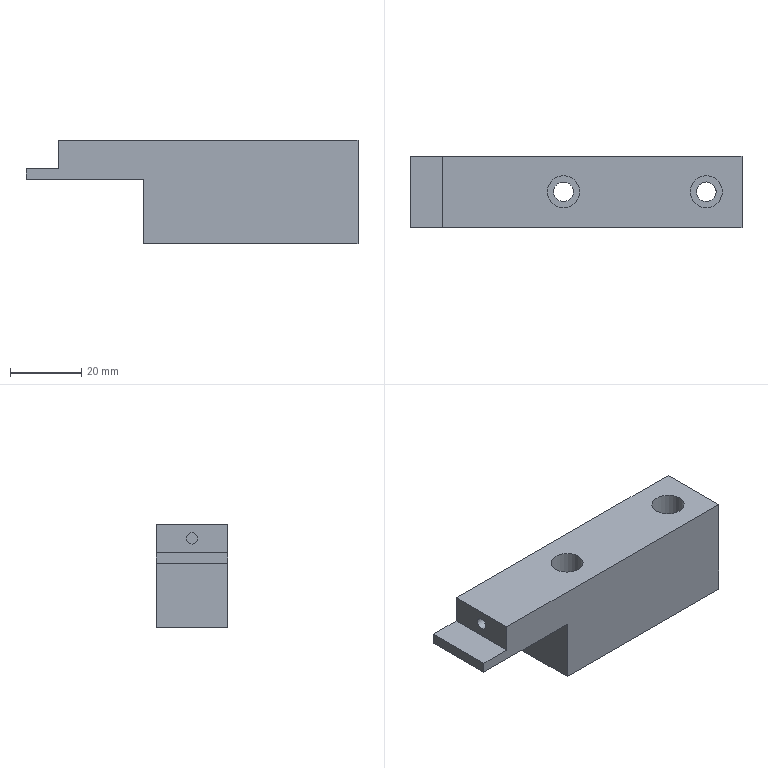Part | NX | 1 solid | 18 faces | box 93 x 20 x 29 mm | volume 38358 mm3 | plane 13 | cylinder 5 | commonest cylinder face diameters 5.5 x2 9 x2 3.2 x1
STEP:
#1=CARTESIAN_POINT('',(744.694,683.943,-134.9));
#2=VERTEX_POINT('',#1);
#3=CARTESIAN_POINT('',(744.694,683.943,-133.3));
#4=DIRECTION('',(1.,0.,0.));
#5=DIRECTION('',(0.,0.,-1.));
#6=AXIS2_PLACEMENT_3D('',#3,#4,#5);
#7=CIRCLE('',#6,1.6);
#8=EDGE_CURVE('',#2,#2,#7,.T.);
#9=ORIENTED_EDGE('',*,*,#8,.F.);
#10=EDGE_LOOP('',(#9));
#11=FACE_BOUND('',#10,.T.);
#12=CARTESIAN_POINT('',(754.694,683.943,-134.9));
#13=VERTEX_POINT('',#12);
#14=CARTESIAN_POINT('',(754.694,683.943,-133.3));
#15=DIRECTION('',(1.,0.,0.));
#16=DIRECTION('',(0.,0.,-1.));
#17=AXIS2_PLACEMENT_3D('',#14,#15,#16);
#18=CIRCLE('',#17,1.6);
#19=EDGE_CURVE('',#13,#13,#18,.T.);
#20=ORIENTED_EDGE('',*,*,#19,.T.);
#21=EDGE_LOOP('',(#20));
#22=FACE_BOUND('',#21,.T.);
#23=CARTESIAN_POINT('',(744.694,683.943,-133.3));
#24=DIRECTION('',(1.,0.,0.));
#25=DIRECTION('',(0.,0.,-1.));
#26=AXIS2_PLACEMENT_3D('',#23,#24,#25);
#27=CYLINDRICAL_SURFACE('',#26,1.6);
#28=ADVANCED_FACE('',(#11,#22),#27,.F.);
#29=ORIENTED_EDGE('',*,*,#19,.F.);
#30=EDGE_LOOP('',(#29));
#31=FACE_BOUND('',#30,.T.);
#32=CARTESIAN_POINT('',(754.694,683.943,-133.3));
#33=DIRECTION('',(1.,0.,0.));
#34=DIRECTION('',(0.,0.,-1.));
#35=AXIS2_PLACEMENT_3D('',#32,#33,#34);
#36=PLANE('',#35);
#37=ADVANCED_FACE('',(#31),#36,.F.);
#38=CARTESIAN_POINT('',(814.094,683.993,-129.35));
#39=VERTEX_POINT('',#38);
#40=CARTESIAN_POINT('',(818.594,683.993,-129.35));
#41=DIRECTION('',(0.,0.,-1.));
#42=DIRECTION('',(-1.,0.,0.));
#43=AXIS2_PLACEMENT_3D('',#40,#41,#42);
#44=CIRCLE('',#43,4.5);
#45=EDGE_CURVE('',#39,#39,#44,.T.);
#46=ORIENTED_EDGE('',*,*,#45,.F.);
#47=EDGE_LOOP('',(#46));
#48=FACE_BOUND('',#47,.T.);
#49=CARTESIAN_POINT('',(814.094,683.993,-139.35));
#50=VERTEX_POINT('',#49);
#51=CARTESIAN_POINT('',(818.594,683.993,-139.35));
#52=DIRECTION('',(0.,0.,-1.));
#53=DIRECTION('',(-1.,0.,0.));
#54=AXIS2_PLACEMENT_3D('',#51,#52,#53);
#55=CIRCLE('',#54,4.5);
#56=EDGE_CURVE('',#50,#50,#55,.T.);
#57=ORIENTED_EDGE('',*,*,#56,.T.);
#58=EDGE_LOOP('',(#57));
#59=FACE_BOUND('',#58,.T.);
#60=CARTESIAN_POINT('',(818.594,683.993,-129.35));
#61=DIRECTION('',(0.,0.,-1.));
#62=DIRECTION('',(-1.,0.,0.));
#63=AXIS2_PLACEMENT_3D('',#60,#61,#62);
#64=CYLINDRICAL_SURFACE('',#63,4.5);
#65=ADVANCED_FACE('',(#48,#59),#64,.F.);
#66=CARTESIAN_POINT('',(818.594,681.243,-139.35));
#67=VERTEX_POINT('',#66);
#68=CARTESIAN_POINT('',(818.594,683.993,-139.35));
#69=DIRECTION('',(0.,0.,1.));
#70=DIRECTION('',(0.,-1.,0.));
#71=AXIS2_PLACEMENT_3D('',#68,#69,#70);
#72=CIRCLE('',#71,2.75);
#73=EDGE_CURVE('',#67,#67,#72,.T.);
#74=ORIENTED_EDGE('',*,*,#73,.F.);
#75=EDGE_LOOP('',(#74));
#76=FACE_BOUND('',#75,.T.);
#77=ORIENTED_EDGE('',*,*,#56,.F.);
#78=EDGE_LOOP('',(#77));
#79=FACE_BOUND('',#78,.T.);
#80=CARTESIAN_POINT('',(818.594,683.993,-139.35));
#81=DIRECTION('',(0.,0.,-1.));
#82=DIRECTION('',(0.,-1.,0.));
#83=AXIS2_PLACEMENT_3D('',#80,#81,#82);
#84=PLANE('',#83);
#85=ADVANCED_FACE('',(#76,#79),#84,.F.);
#86=CARTESIAN_POINT('',(774.094,683.993,-129.35));
#87=VERTEX_POINT('',#86);
#88=CARTESIAN_POINT('',(778.594,683.993,-129.35));
#89=DIRECTION('',(0.,0.,-1.));
#90=DIRECTION('',(-1.,0.,0.));
#91=AXIS2_PLACEMENT_3D('',#88,#89,#90);
#92=CIRCLE('',#91,4.5);
#93=EDGE_CURVE('',#87,#87,#92,.T.);
#94=ORIENTED_EDGE('',*,*,#93,.F.);
#95=EDGE_LOOP('',(#94));
#96=FACE_BOUND('',#95,.T.);
#97=CARTESIAN_POINT('',(774.094,683.993,-139.35));
#98=VERTEX_POINT('',#97);
#99=CARTESIAN_POINT('',(778.594,683.993,-139.35));
#100=DIRECTION('',(0.,0.,-1.));
#101=DIRECTION('',(-1.,0.,0.));
#102=AXIS2_PLACEMENT_3D('',#99,#100,#101);
#103=CIRCLE('',#102,4.5);
#104=EDGE_CURVE('',#98,#98,#103,.T.);
#105=ORIENTED_EDGE('',*,*,#104,.T.);
#106=EDGE_LOOP('',(#105));
#107=FACE_BOUND('',#106,.T.);
#108=CARTESIAN_POINT('',(778.594,683.993,-129.35));
#109=DIRECTION('',(0.,0.,-1.));
#110=DIRECTION('',(-1.,0.,0.));
#111=AXIS2_PLACEMENT_3D('',#108,#109,#110);
#112=CYLINDRICAL_SURFACE('',#111,4.5);
#113=ADVANCED_FACE('',(#96,#107),#112,.F.);
#114=CARTESIAN_POINT('',(775.844,683.993,-139.35));
#115=VERTEX_POINT('',#114);
#116=CARTESIAN_POINT('',(778.594,683.993,-139.35));
#117=DIRECTION('',(0.,0.,1.));
#118=DIRECTION('',(-1.,0.,0.));
#119=AXIS2_PLACEMENT_3D('',#116,#117,#118);
#120=CIRCLE('',#119,2.75);
#121=EDGE_CURVE('',#115,#115,#120,.T.);
#122=ORIENTED_EDGE('',*,*,#121,.F.);
#123=EDGE_LOOP('',(#122));
#124=FACE_BOUND('',#123,.T.);
#125=ORIENTED_EDGE('',*,*,#104,.F.);
#126=EDGE_LOOP('',(#125));
#127=FACE_BOUND('',#126,.T.);
#128=CARTESIAN_POINT('',(818.594,683.993,-139.35));
#129=DIRECTION('',(0.,0.,-1.));
#130=DIRECTION('',(0.,-1.,0.));
#131=AXIS2_PLACEMENT_3D('',#128,#129,#130);
#132=PLANE('',#131);
#133=ADVANCED_FACE('',(#124,#127),#132,.F.);
#134=CARTESIAN_POINT('',(781.344,683.993,-158.35));
#135=VERTEX_POINT('',#134);
#136=CARTESIAN_POINT('',(778.594,683.993,-158.35));
#137=DIRECTION('',(0.,0.,-1.));
#138=DIRECTION('',(1.,0.,0.));
#139=AXIS2_PLACEMENT_3D('',#136,#137,#138);
#140=CIRCLE('',#139,2.75);
#141=EDGE_CURVE('',#135,#135,#140,.T.);
#142=ORIENTED_EDGE('',*,*,#141,.T.);
#143=EDGE_LOOP('',(#142));
#144=FACE_BOUND('',#143,.T.);
#145=ORIENTED_EDGE('',*,*,#121,.T.);
#146=EDGE_LOOP('',(#145));
#147=FACE_BOUND('',#146,.T.);
#148=CARTESIAN_POINT('',(778.594,683.993,-157.35));
#149=DIRECTION('',(0.,0.,1.));
#150=DIRECTION('',(1.,0.,0.));
#151=AXIS2_PLACEMENT_3D('',#148,#149,#150);
#152=CYLINDRICAL_SURFACE('',#151,2.75);
#153=ADVANCED_FACE('',(#144,#147),#152,.F.);
#154=CARTESIAN_POINT('',(821.344,683.993,-158.35));
#155=VERTEX_POINT('',#154);
#156=CARTESIAN_POINT('',(818.594,683.993,-158.35));
#157=DIRECTION('',(0.,0.,1.));
#158=DIRECTION('',(1.,0.,0.));
#159=AXIS2_PLACEMENT_3D('',#156,#157,#158);
#160=CIRCLE('',#159,2.75);
#161=EDGE_CURVE('',#155,#155,#160,.T.);
#162=ORIENTED_EDGE('',*,*,#161,.F.);
#163=EDGE_LOOP('',(#162));
#164=FACE_BOUND('',#163,.T.);
#165=ORIENTED_EDGE('',*,*,#73,.T.);
#166=EDGE_LOOP('',(#165));
#167=FACE_BOUND('',#166,.T.);
#168=CARTESIAN_POINT('',(818.594,683.993,-157.35));
#169=DIRECTION('',(0.,0.,1.));
#170=DIRECTION('',(-1.,0.,0.));
#171=AXIS2_PLACEMENT_3D('',#168,#169,#170);
#172=CYLINDRICAL_SURFACE('',#171,2.75);
#173=ADVANCED_FACE('',(#164,#167),#172,.F.);
#174=CARTESIAN_POINT('',(744.694,673.943,-129.35));
#175=VERTEX_POINT('',#174);
#176=CARTESIAN_POINT('',(744.694,673.943,-137.3));
#177=VERTEX_POINT('',#176);
#178=CARTESIAN_POINT('',(744.694,673.943,-129.35));
#179=DIRECTION('',(0.,0.,-1.));
#180=VECTOR('',#179,1000.);
#181=LINE('',#178,#180);
#182=EDGE_CURVE('',#175,#177,#181,.T.);
#183=ORIENTED_EDGE('',*,*,#182,.F.);
#184=CARTESIAN_POINT('',(744.694,693.943,-129.35));
#185=VERTEX_POINT('',#184);
#186=CARTESIAN_POINT('',(744.694,892.443,-129.35));
#187=DIRECTION('',(0.,-1.,0.));
#188=VECTOR('',#187,1000.);
#189=LINE('',#186,#188);
#190=EDGE_CURVE('',#185,#175,#189,.T.);
#191=ORIENTED_EDGE('',*,*,#190,.F.);
#192=CARTESIAN_POINT('',(744.694,693.943,-137.3));
#193=VERTEX_POINT('',#192);
#194=CARTESIAN_POINT('',(744.694,693.943,-129.35));
#195=DIRECTION('',(0.,0.,-1.));
#196=VECTOR('',#195,1000.);
#197=LINE('',#194,#196);
#198=EDGE_CURVE('',#185,#193,#197,.T.);
#199=ORIENTED_EDGE('',*,*,#198,.T.);
#200=CARTESIAN_POINT('',(744.694,892.443,-137.3));
#201=DIRECTION('',(0.,1.,0.));
#202=VECTOR('',#201,1000.);
#203=LINE('',#200,#202);
#204=EDGE_CURVE('',#177,#193,#203,.T.);
#205=ORIENTED_EDGE('',*,*,#204,.F.);
#206=EDGE_LOOP('',(#183,#191,#199,#205));
#207=FACE_BOUND('',#206,.T.);
#208=ORIENTED_EDGE('',*,*,#8,.T.);
#209=EDGE_LOOP('',(#208));
#210=FACE_BOUND('',#209,.T.);
#211=CARTESIAN_POINT('',(744.694,892.443,-139.3));
#212=DIRECTION('',(1.,0.,0.));
#213=DIRECTION('',(0.,1.,0.));
#214=AXIS2_PLACEMENT_3D('',#211,#212,#213);
#215=PLANE('',#214);
#216=ADVANCED_FACE('',(#207,#210),#215,.F.);
#217=CARTESIAN_POINT('',(768.594,693.943,-140.35));
#218=VERTEX_POINT('',#217);
#219=CARTESIAN_POINT('',(768.594,673.943,-140.35));
#220=VERTEX_POINT('',#219);
#221=CARTESIAN_POINT('',(768.594,605.243,-140.35));
#222=DIRECTION('',(0.,-1.,0.));
#223=VECTOR('',#222,1000.);
#224=LINE('',#221,#223);
#225=EDGE_CURVE('',#218,#220,#224,.T.);
#226=ORIENTED_EDGE('',*,*,#225,.F.);
#227=CARTESIAN_POINT('',(768.594,693.943,-158.35));
#228=VERTEX_POINT('',#227);
#229=CARTESIAN_POINT('',(768.594,693.943,-164.35));
#230=DIRECTION('',(0.,0.,-1.));
#231=VECTOR('',#230,1000.);
#232=LINE('',#229,#231);
#233=EDGE_CURVE('',#218,#228,#232,.T.);
#234=ORIENTED_EDGE('',*,*,#233,.T.);
#235=CARTESIAN_POINT('',(768.594,673.943,-158.35));
#236=VERTEX_POINT('',#235);
#237=CARTESIAN_POINT('',(768.594,605.243,-158.35));
#238=DIRECTION('',(0.,1.,0.));
#239=VECTOR('',#238,1000.);
#240=LINE('',#237,#239);
#241=EDGE_CURVE('',#236,#228,#240,.T.);
#242=ORIENTED_EDGE('',*,*,#241,.F.);
#243=CARTESIAN_POINT('',(768.594,673.943,-164.35));
#244=DIRECTION('',(0.,0.,-1.));
#245=VECTOR('',#244,1000.);
#246=LINE('',#243,#245);
#247=EDGE_CURVE('',#220,#236,#246,.T.);
#248=ORIENTED_EDGE('',*,*,#247,.F.);
#249=EDGE_LOOP('',(#226,#234,#242,#248));
#250=FACE_BOUND('',#249,.T.);
#251=CARTESIAN_POINT('',(768.594,605.243,-164.35));
#252=DIRECTION('',(-1.,0.,0.));
#253=DIRECTION('',(0.,-1.,0.));
#254=AXIS2_PLACEMENT_3D('',#251,#252,#253);
#255=PLANE('',#254);
#256=ADVANCED_FACE('',(#250),#255,.T.);
#257=ORIENTED_EDGE('',*,*,#241,.T.);
#258=CARTESIAN_POINT('',(828.594,693.943,-158.35));
#259=VERTEX_POINT('',#258);
#260=CARTESIAN_POINT('',(798.594,693.943,-158.35));
#261=DIRECTION('',(1.,0.,0.));
#262=VECTOR('',#261,1000.);
#263=LINE('',#260,#262);
#264=EDGE_CURVE('',#228,#259,#263,.T.);
#265=ORIENTED_EDGE('',*,*,#264,.T.);
#266=CARTESIAN_POINT('',(828.594,673.943,-158.35));
#267=VERTEX_POINT('',#266);
#268=CARTESIAN_POINT('',(828.594,605.243,-158.35));
#269=DIRECTION('',(0.,1.,0.));
#270=VECTOR('',#269,1000.);
#271=LINE('',#268,#270);
#272=EDGE_CURVE('',#267,#259,#271,.T.);
#273=ORIENTED_EDGE('',*,*,#272,.F.);
#274=CARTESIAN_POINT('',(798.594,673.943,-158.35));
#275=DIRECTION('',(1.,0.,0.));
#276=VECTOR('',#275,1000.);
#277=LINE('',#274,#276);
#278=EDGE_CURVE('',#236,#267,#277,.T.);
#279=ORIENTED_EDGE('',*,*,#278,.F.);
#280=EDGE_LOOP('',(#257,#265,#273,#279));
#281=FACE_BOUND('',#280,.T.);
#282=ORIENTED_EDGE('',*,*,#161,.T.);
#283=EDGE_LOOP('',(#282));
#284=FACE_BOUND('',#283,.T.);
#285=ORIENTED_EDGE('',*,*,#141,.F.);
#286=EDGE_LOOP('',(#285));
#287=FACE_BOUND('',#286,.T.);
#288=CARTESIAN_POINT('',(798.594,605.243,-158.35));
#289=DIRECTION('',(0.,0.,1.));
#290=DIRECTION('',(0.,1.,0.));
#291=AXIS2_PLACEMENT_3D('',#288,#289,#290);
#292=PLANE('',#291);
#293=ADVANCED_FACE('',(#281,#284,#287),#292,.F.);
#294=CARTESIAN_POINT('',(735.594,693.943,-137.3));
#295=VERTEX_POINT('',#294);
#296=CARTESIAN_POINT('',(830.394,693.943,-137.3));
#297=DIRECTION('',(-1.,0.,0.));
#298=VECTOR('',#297,1000.);
#299=LINE('',#296,#298);
#300=EDGE_CURVE('',#193,#295,#299,.T.);
#301=ORIENTED_EDGE('',*,*,#300,.T.);
#302=CARTESIAN_POINT('',(735.594,673.943,-137.3));
#303=VERTEX_POINT('',#302);
#304=CARTESIAN_POINT('',(735.594,717.943,-137.3));
#305=DIRECTION('',(0.,1.,0.));
#306=VECTOR('',#305,1000.);
#307=LINE('',#304,#306);
#308=EDGE_CURVE('',#303,#295,#307,.T.);
#309=ORIENTED_EDGE('',*,*,#308,.F.);
#310=CARTESIAN_POINT('',(830.394,673.943,-137.3));
#311=DIRECTION('',(-1.,0.,0.));
#312=VECTOR('',#311,1000.);
#313=LINE('',#310,#312);
#314=EDGE_CURVE('',#177,#303,#313,.T.);
#315=ORIENTED_EDGE('',*,*,#314,.F.);
#316=ORIENTED_EDGE('',*,*,#204,.T.);
#317=EDGE_LOOP('',(#301,#309,#315,#316));
#318=FACE_BOUND('',#317,.T.);
#319=CARTESIAN_POINT('',(743.694,717.943,-137.3));
#320=DIRECTION('',(0.,0.,-1.));
#321=DIRECTION('',(0.,-1.,0.));
#322=AXIS2_PLACEMENT_3D('',#319,#320,#321);
#323=PLANE('',#322);
#324=ADVANCED_FACE('',(#318),#323,.F.);
#325=CARTESIAN_POINT('',(828.594,673.943,-129.35));
#326=VERTEX_POINT('',#325);
#327=CARTESIAN_POINT('',(828.594,673.943,-129.35));
#328=DIRECTION('',(0.,0.,-1.));
#329=VECTOR('',#328,1000.);
#330=LINE('',#327,#329);
#331=EDGE_CURVE('',#326,#267,#330,.T.);
#332=ORIENTED_EDGE('',*,*,#331,.T.);
#333=ORIENTED_EDGE('',*,*,#272,.T.);
#334=CARTESIAN_POINT('',(828.594,693.943,-129.35));
#335=VERTEX_POINT('',#334);
#336=CARTESIAN_POINT('',(828.594,693.943,-164.35));
#337=DIRECTION('',(0.,0.,1.));
#338=VECTOR('',#337,1000.);
#339=LINE('',#336,#338);
#340=EDGE_CURVE('',#259,#335,#339,.T.);
#341=ORIENTED_EDGE('',*,*,#340,.T.);
#342=CARTESIAN_POINT('',(828.594,570.943,-129.35));
#343=DIRECTION('',(0.,1.,0.));
#344=VECTOR('',#343,1000.);
#345=LINE('',#342,#344);
#346=EDGE_CURVE('',#326,#335,#345,.T.);
#347=ORIENTED_EDGE('',*,*,#346,.F.);
#348=EDGE_LOOP('',(#332,#333,#341,#347));
#349=FACE_BOUND('',#348,.T.);
#350=CARTESIAN_POINT('',(828.594,605.243,-164.35));
#351=DIRECTION('',(1.,0.,0.));
#352=DIRECTION('',(0.,1.,0.));
#353=AXIS2_PLACEMENT_3D('',#350,#351,#352);
#354=PLANE('',#353);
#355=ADVANCED_FACE('',(#349),#354,.T.);
#356=CARTESIAN_POINT('',(830.394,673.943,-129.35));
#357=DIRECTION('',(1.,0.,0.));
#358=VECTOR('',#357,1000.);
#359=LINE('',#356,#358);
#360=EDGE_CURVE('',#175,#326,#359,.T.);
#361=ORIENTED_EDGE('',*,*,#360,.F.);
#362=ORIENTED_EDGE('',*,*,#182,.T.);
#363=ORIENTED_EDGE('',*,*,#314,.T.);
#364=CARTESIAN_POINT('',(735.594,673.943,-140.35));
#365=VERTEX_POINT('',#364);
#366=CARTESIAN_POINT('',(735.594,673.943,-139.3));
#367=DIRECTION('',(0.,0.,-1.));
#368=VECTOR('',#367,1000.);
#369=LINE('',#366,#368);
#370=EDGE_CURVE('',#303,#365,#369,.T.);
#371=ORIENTED_EDGE('',*,*,#370,.T.);
#372=CARTESIAN_POINT('',(740.194,673.943,-140.35));
#373=DIRECTION('',(1.,0.,0.));
#374=VECTOR('',#373,1000.);
#375=LINE('',#372,#374);
#376=EDGE_CURVE('',#365,#220,#375,.T.);
#377=ORIENTED_EDGE('',*,*,#376,.T.);
#378=ORIENTED_EDGE('',*,*,#247,.T.);
#379=ORIENTED_EDGE('',*,*,#278,.T.);
#380=ORIENTED_EDGE('',*,*,#331,.F.);
#381=EDGE_LOOP('',(#361,#362,#363,#371,#377,#378,#379,#380));
#382=FACE_BOUND('',#381,.T.);
#383=CARTESIAN_POINT('',(830.394,673.943,-129.35));
#384=DIRECTION('',(0.,1.,0.));
#385=DIRECTION('',(-1.,0.,0.));
#386=AXIS2_PLACEMENT_3D('',#383,#384,#385);
#387=PLANE('',#386);
#388=ADVANCED_FACE('',(#382),#387,.F.);
#389=ORIENTED_EDGE('',*,*,#300,.F.);
#390=ORIENTED_EDGE('',*,*,#198,.F.);
#391=CARTESIAN_POINT('',(830.394,693.943,-129.35));
#392=DIRECTION('',(1.,0.,0.));
#393=VECTOR('',#392,1000.);
#394=LINE('',#391,#393);
#395=EDGE_CURVE('',#185,#335,#394,.T.);
#396=ORIENTED_EDGE('',*,*,#395,.T.);
#397=ORIENTED_EDGE('',*,*,#340,.F.);
#398=ORIENTED_EDGE('',*,*,#264,.F.);
#399=ORIENTED_EDGE('',*,*,#233,.F.);
#400=CARTESIAN_POINT('',(735.594,693.943,-140.35));
#401=VERTEX_POINT('',#400);
#402=CARTESIAN_POINT('',(830.394,693.943,-140.35));
#403=DIRECTION('',(-1.,0.,0.));
#404=VECTOR('',#403,1000.);
#405=LINE('',#402,#404);
#406=EDGE_CURVE('',#218,#401,#405,.T.);
#407=ORIENTED_EDGE('',*,*,#406,.T.);
#408=CARTESIAN_POINT('',(735.594,693.943,-139.3));
#409=DIRECTION('',(0.,0.,-1.));
#410=VECTOR('',#409,1000.);
#411=LINE('',#408,#410);
#412=EDGE_CURVE('',#295,#401,#411,.T.);
#413=ORIENTED_EDGE('',*,*,#412,.F.);
#414=EDGE_LOOP('',(#389,#390,#396,#397,#398,#399,#407,#413));
#415=FACE_BOUND('',#414,.T.);
#416=CARTESIAN_POINT('',(830.394,693.943,-129.35));
#417=DIRECTION('',(0.,1.,0.));
#418=DIRECTION('',(-1.,0.,0.));
#419=AXIS2_PLACEMENT_3D('',#416,#417,#418);
#420=PLANE('',#419);
#421=ADVANCED_FACE('',(#415),#420,.T.);
#422=ORIENTED_EDGE('',*,*,#412,.T.);
#423=CARTESIAN_POINT('',(735.594,683.943,-140.35));
#424=DIRECTION('',(0.,1.,0.));
#425=VECTOR('',#424,1000.);
#426=LINE('',#423,#425);
#427=EDGE_CURVE('',#365,#401,#426,.T.);
#428=ORIENTED_EDGE('',*,*,#427,.F.);
#429=ORIENTED_EDGE('',*,*,#370,.F.);
#430=ORIENTED_EDGE('',*,*,#308,.T.);
#431=EDGE_LOOP('',(#422,#428,#429,#430));
#432=FACE_BOUND('',#431,.T.);
#433=CARTESIAN_POINT('',(735.594,887.943,-139.3));
#434=DIRECTION('',(1.,0.,0.));
#435=DIRECTION('',(0.,1.,0.));
#436=AXIS2_PLACEMENT_3D('',#433,#434,#435);
#437=PLANE('',#436);
#438=ADVANCED_FACE('',(#432),#437,.F.);
#439=ORIENTED_EDGE('',*,*,#406,.F.);
#440=ORIENTED_EDGE('',*,*,#225,.T.);
#441=ORIENTED_EDGE('',*,*,#376,.F.);
#442=ORIENTED_EDGE('',*,*,#427,.T.);
#443=EDGE_LOOP('',(#439,#440,#441,#442));
#444=FACE_BOUND('',#443,.T.);
#445=CARTESIAN_POINT('',(740.194,683.943,-140.35));
#446=DIRECTION('',(0.,0.,-1.));
#447=DIRECTION('',(0.,-1.,0.));
#448=AXIS2_PLACEMENT_3D('',#445,#446,#447);
#449=PLANE('',#448);
#450=ADVANCED_FACE('',(#444),#449,.T.);
#451=ORIENTED_EDGE('',*,*,#395,.F.);
#452=ORIENTED_EDGE('',*,*,#190,.T.);
#453=ORIENTED_EDGE('',*,*,#360,.T.);
#454=ORIENTED_EDGE('',*,*,#346,.T.);
#455=EDGE_LOOP('',(#451,#452,#453,#454));
#456=FACE_BOUND('',#455,.T.);
#457=ORIENTED_EDGE('',*,*,#93,.T.);
#458=EDGE_LOOP('',(#457));
#459=FACE_BOUND('',#458,.T.);
#460=ORIENTED_EDGE('',*,*,#45,.T.);
#461=EDGE_LOOP('',(#460));
#462=FACE_BOUND('',#461,.T.);
#463=CARTESIAN_POINT('',(795.194,570.943,-129.35));
#464=DIRECTION('',(0.,0.,1.));
#465=DIRECTION('',(0.,1.,0.));
#466=AXIS2_PLACEMENT_3D('',#463,#464,#465);
#467=PLANE('',#466);
#468=ADVANCED_FACE('',(#456,#459,#462),#467,.T.);
#469=CLOSED_SHELL('',(#28,#37,#65,#85,#113,#133,#153,#173,#216,#256,#293,#324,#355,#388,#421,#438,#450,#468));
#470=MANIFOLD_SOLID_BREP('',#469);
#471=(LENGTH_UNIT()NAMED_UNIT(*)SI_UNIT(.MILLI.,.METRE.));
#472=UNCERTAINTY_MEASURE_WITH_UNIT(LENGTH_MEASURE(0.00001),#471,'','');
#473=(NAMED_UNIT(*)PLANE_ANGLE_UNIT()SI_UNIT($,.RADIAN.));
#474=(NAMED_UNIT(*)SI_UNIT($,.STERADIAN.)SOLID_ANGLE_UNIT());
#475=(GEOMETRIC_REPRESENTATION_CONTEXT(3)GLOBAL_UNCERTAINTY_ASSIGNED_CONTEXT((#472))GLOBAL_UNIT_ASSIGNED_CONTEXT((#471,#473,#474))REPRESENTATION_CONTEXT('',''));
#476=ADVANCED_BREP_SHAPE_REPRESENTATION('',(#470),#475);